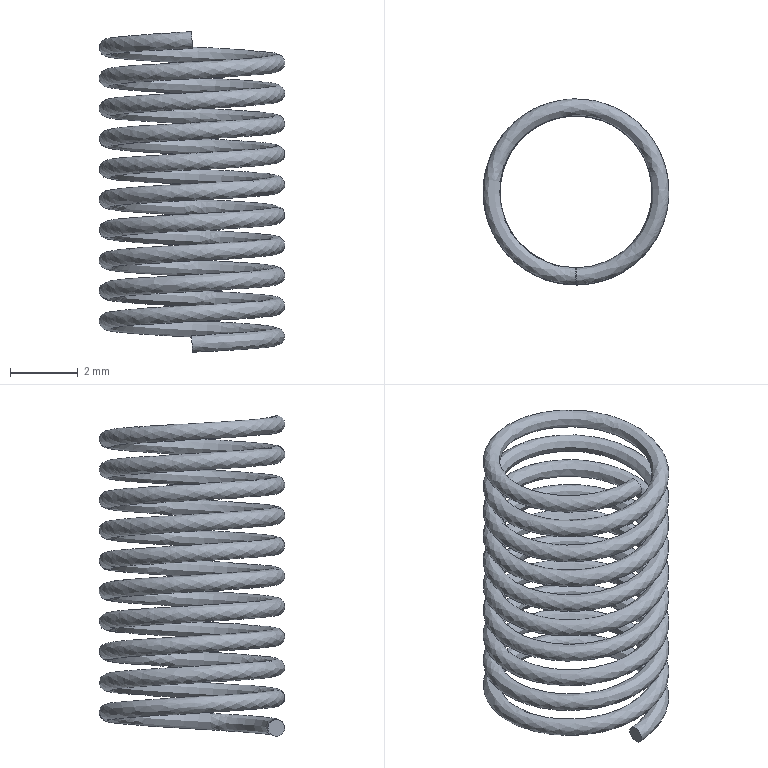Part | STEP file | 1-67.2 | 1 solid | 3 faces | box 5.501 x 5.5 x 9.499 mm | volume 30.865 mm3 | plane 2 | spline 1